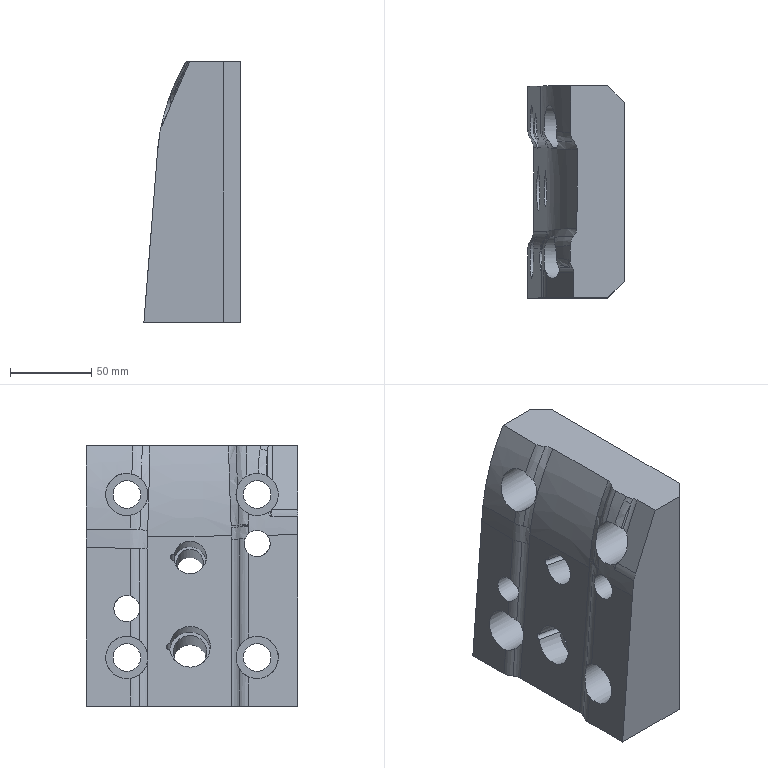Part | NX | features solid 2 | 1 solid | 67 faces | box 59.098 x 130 x 160 mm | volume 873693 mm3 | cylinder 30 | plane 20 | spline 17 | commonest cylinder face diameters 20 x6 16 x5 17 x4 26 x4 4 x2 10 x1